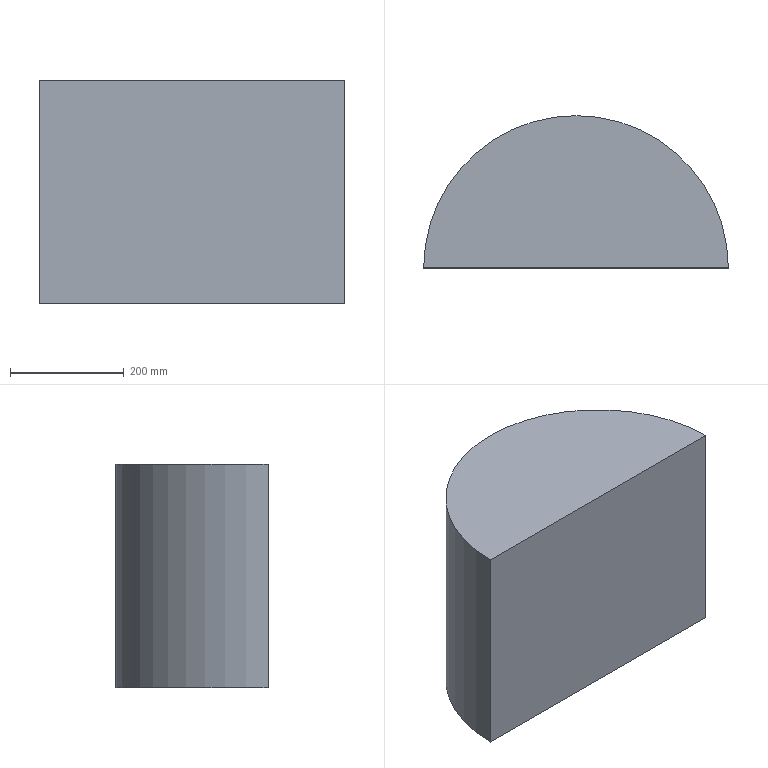Part | STEP file | Boss-Extrude 47 | 1 solid | 4 faces | box 536.8 x 268.4 x 393 mm | volume 44471057 mm3 | plane 3 | cylinder 1 | commonest cylinder face diameters 536.8 x1
STEP:
#1=CARTESIAN_POINT('',(-480.338,-924.736,2973.5));
#2=VERTEX_POINT('',#1);
#3=CARTESIAN_POINT('',(-1017.138,-924.736,2973.5));
#4=VERTEX_POINT('',#3);
#5=CARTESIAN_POINT('',(-748.738,-924.736,2973.5));
#6=DIRECTION('',(0.,0.,1.));
#7=DIRECTION('',(1.,0.,0.));
#8=AXIS2_PLACEMENT_3D('',#5,#6,#7);
#9=CIRCLE('',#8,268.4);
#10=EDGE_CURVE('',#2,#4,#9,.T.);
#11=ORIENTED_EDGE('',*,*,#10,.F.);
#12=CARTESIAN_POINT('',(-480.338,-924.736,2580.5));
#13=VERTEX_POINT('',#12);
#14=CARTESIAN_POINT('',(-480.338,-924.736,2580.5));
#15=DIRECTION('',(0.,0.,1.));
#16=VECTOR('',#15,1000.);
#17=LINE('',#14,#16);
#18=EDGE_CURVE('',#13,#2,#17,.T.);
#19=ORIENTED_EDGE('',*,*,#18,.F.);
#20=CARTESIAN_POINT('',(-1017.138,-924.736,2580.5));
#21=VERTEX_POINT('',#20);
#22=CARTESIAN_POINT('',(-748.738,-924.736,2580.5));
#23=DIRECTION('',(0.,0.,1.));
#24=DIRECTION('',(1.,0.,0.));
#25=AXIS2_PLACEMENT_3D('',#22,#23,#24);
#26=CIRCLE('',#25,268.4);
#27=EDGE_CURVE('',#13,#21,#26,.T.);
#28=ORIENTED_EDGE('',*,*,#27,.T.);
#29=CARTESIAN_POINT('',(-1017.138,-924.736,2580.5));
#30=DIRECTION('',(0.,0.,1.));
#31=VECTOR('',#30,1000.);
#32=LINE('',#29,#31);
#33=EDGE_CURVE('',#21,#4,#32,.T.);
#34=ORIENTED_EDGE('',*,*,#33,.T.);
#35=EDGE_LOOP('',(#11,#19,#28,#34));
#36=FACE_OUTER_BOUND('',#35,.T.);
#37=CARTESIAN_POINT('',(-748.738,-924.736,2580.5));
#38=DIRECTION('',(0.,0.,1.));
#39=DIRECTION('',(-1.,0.,0.));
#40=AXIS2_PLACEMENT_3D('',#37,#38,#39);
#41=CYLINDRICAL_SURFACE('',#40,268.4);
#42=ADVANCED_FACE('',(#36),#41,.T.);
#43=CARTESIAN_POINT('',(-480.338,-924.736,2973.5));
#44=DIRECTION('',(1.,0.,0.));
#45=VECTOR('',#44,1000.);
#46=LINE('',#43,#45);
#47=EDGE_CURVE('',#4,#2,#46,.T.);
#48=ORIENTED_EDGE('',*,*,#47,.F.);
#49=ORIENTED_EDGE('',*,*,#33,.F.);
#50=CARTESIAN_POINT('',(-480.338,-924.736,2580.5));
#51=DIRECTION('',(1.,0.,0.));
#52=VECTOR('',#51,1000.);
#53=LINE('',#50,#52);
#54=EDGE_CURVE('',#21,#13,#53,.T.);
#55=ORIENTED_EDGE('',*,*,#54,.T.);
#56=ORIENTED_EDGE('',*,*,#18,.T.);
#57=EDGE_LOOP('',(#48,#49,#55,#56));
#58=FACE_OUTER_BOUND('',#57,.T.);
#59=CARTESIAN_POINT('',(-480.338,-924.736,2580.5));
#60=DIRECTION('',(0.,-1.,0.));
#61=DIRECTION('',(-1.,0.,0.));
#62=AXIS2_PLACEMENT_3D('',#59,#60,#61);
#63=PLANE('',#62);
#64=ADVANCED_FACE('',(#58),#63,.T.);
#65=ORIENTED_EDGE('',*,*,#27,.F.);
#66=ORIENTED_EDGE('',*,*,#54,.F.);
#67=EDGE_LOOP('',(#65,#66));
#68=FACE_OUTER_BOUND('',#67,.T.);
#69=CARTESIAN_POINT('',(-748.738,-924.736,2580.5));
#70=DIRECTION('',(0.,0.,1.));
#71=DIRECTION('',(-1.,0.,0.));
#72=AXIS2_PLACEMENT_3D('',#69,#70,#71);
#73=PLANE('',#72);
#74=ADVANCED_FACE('',(#68),#73,.F.);
#75=ORIENTED_EDGE('',*,*,#10,.T.);
#76=ORIENTED_EDGE('',*,*,#47,.T.);
#77=EDGE_LOOP('',(#75,#76));
#78=FACE_OUTER_BOUND('',#77,.T.);
#79=CARTESIAN_POINT('',(-748.738,-924.736,2973.5));
#80=DIRECTION('',(0.,0.,1.));
#81=DIRECTION('',(-1.,0.,0.));
#82=AXIS2_PLACEMENT_3D('',#79,#80,#81);
#83=PLANE('',#82);
#84=ADVANCED_FACE('',(#78),#83,.T.);
#85=CLOSED_SHELL('',(#42,#64,#74,#84));
#86=MANIFOLD_SOLID_BREP('',#85);
#87=CARTESIAN_POINT('',(0.,0.,0.));
#88=DIRECTION('',(0.,0.,1.));
#89=DIRECTION('',(1.,0.,0.));
#90=AXIS2_PLACEMENT_3D('',#87,#88,#89);
#91=(LENGTH_UNIT()NAMED_UNIT(*)SI_UNIT(.MILLI.,.METRE.));
#92=UNCERTAINTY_MEASURE_WITH_UNIT(LENGTH_MEASURE(0.00001),#91,'','');
#93=(NAMED_UNIT(*)PLANE_ANGLE_UNIT()SI_UNIT($,.RADIAN.));
#94=(NAMED_UNIT(*)SI_UNIT($,.STERADIAN.)SOLID_ANGLE_UNIT());
#95=(GEOMETRIC_REPRESENTATION_CONTEXT(3)GLOBAL_UNCERTAINTY_ASSIGNED_CONTEXT((#92))GLOBAL_UNIT_ASSIGNED_CONTEXT((#91,#93,#94))REPRESENTATION_CONTEXT('',''));
#96=ADVANCED_BREP_SHAPE_REPRESENTATION('',(#86,#90),#95);